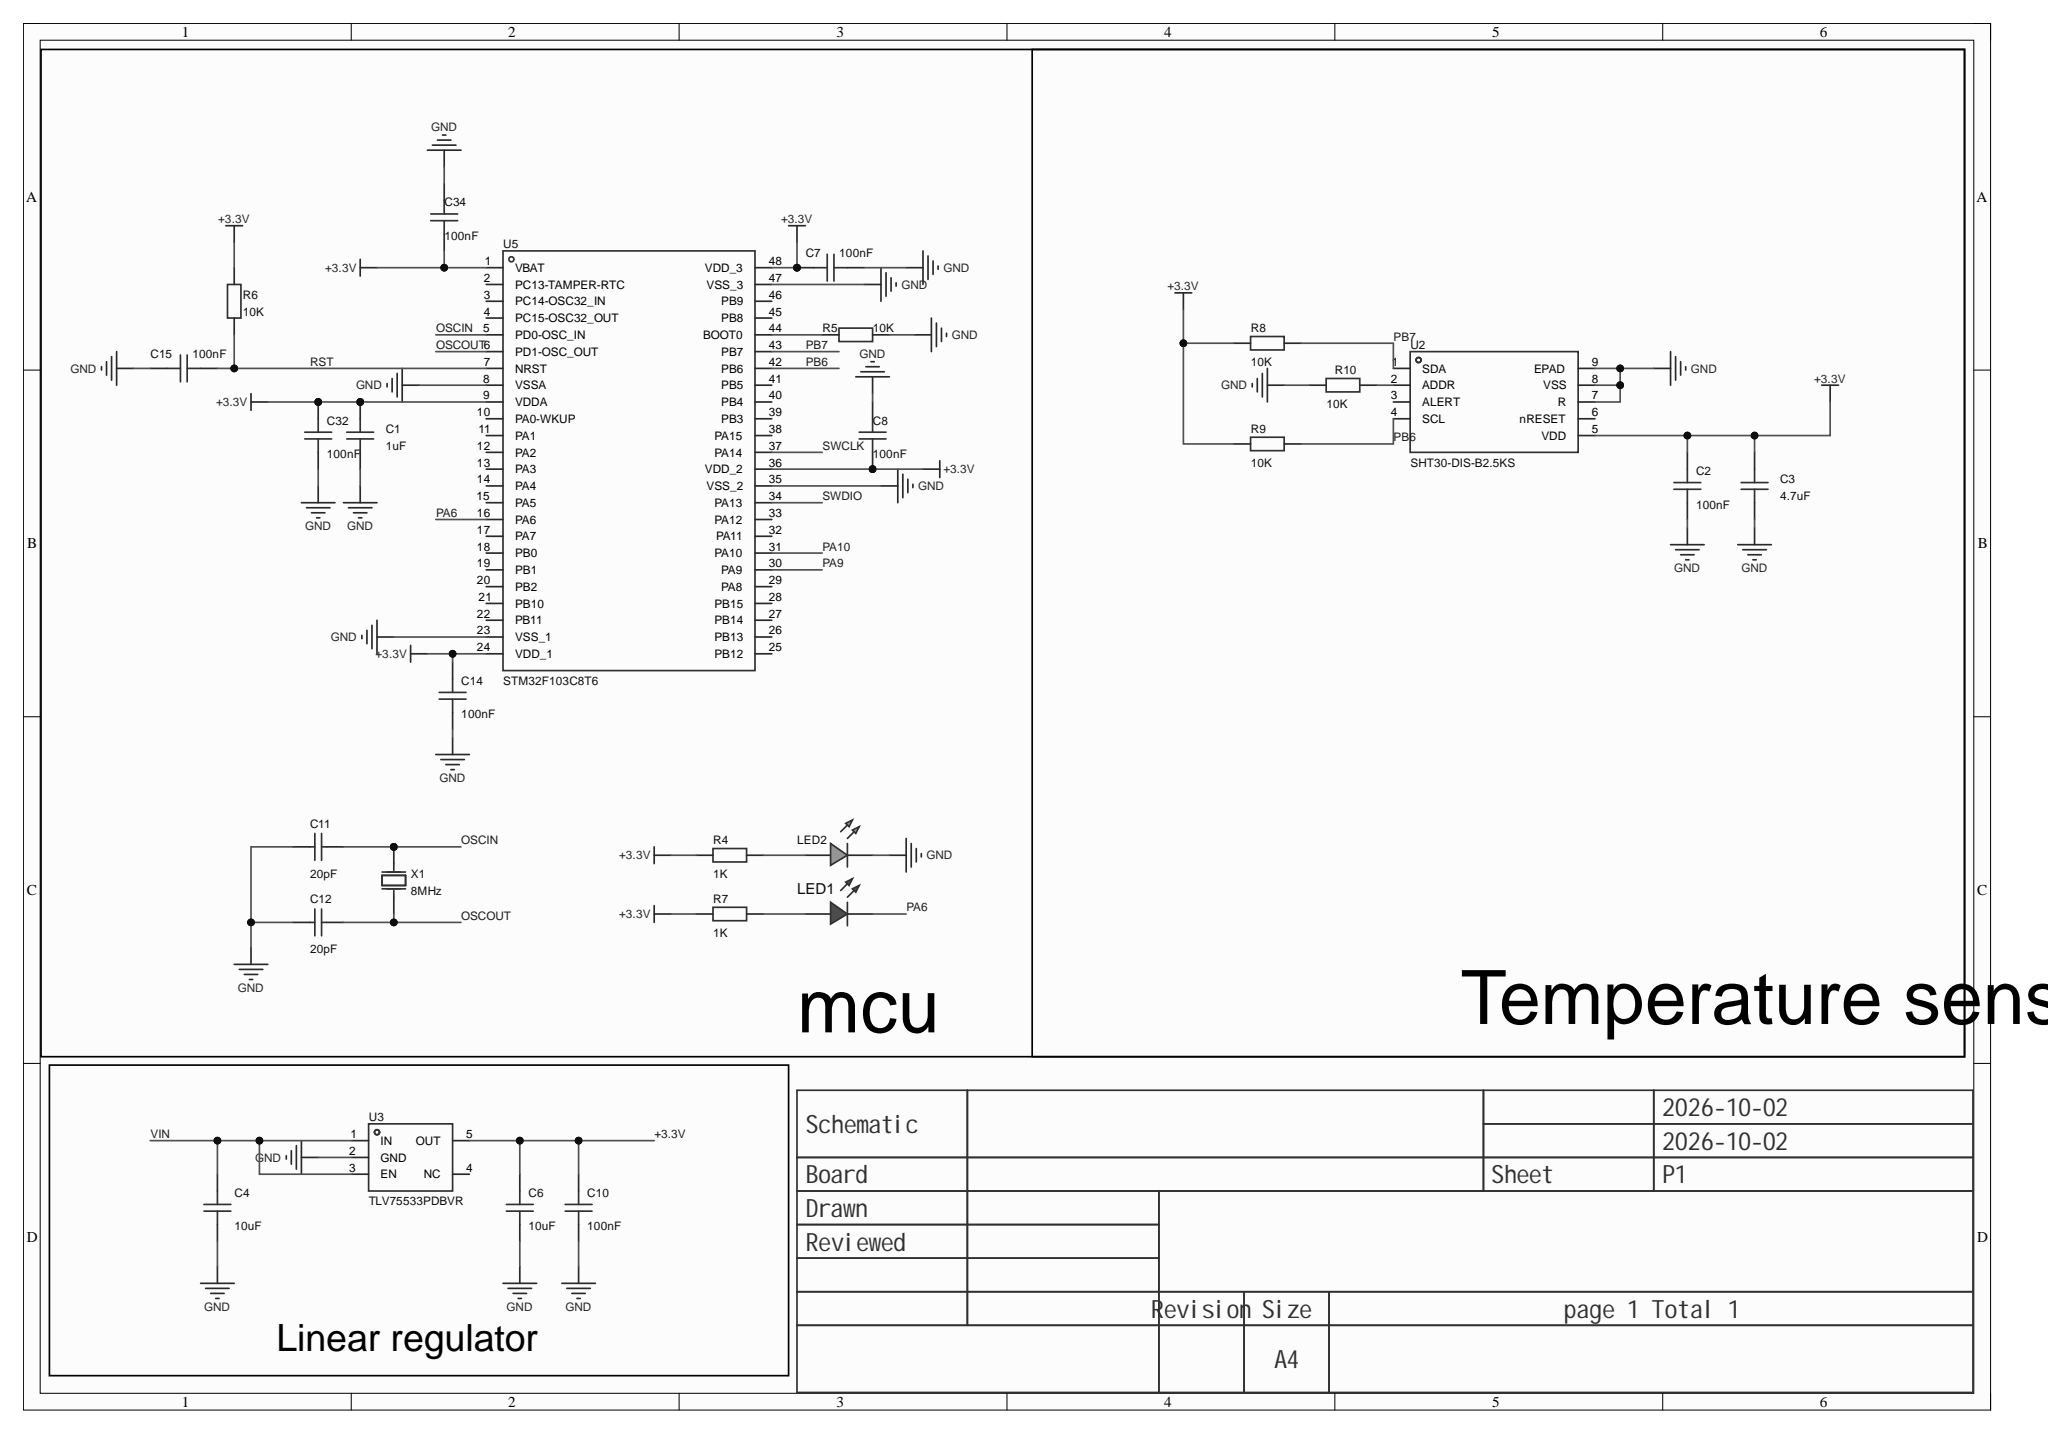Circuit board | Altium Designer | 27 parts | 13 nets
Bill of materials:
Comment,Description,Designator,Footprint,LibRef,Quantity
"1uF","Capacitance:1uF;Accuracy:±10%;Rated voltage:50V;Temperature coefficient:X5R;","C1","C0603","CL10A105KB8NNNC","1"
"100nF","Capacitance:100nF;Accuracy:±10%;Rated voltage:50V;Temperature coefficient:X7R;, [NoValue]","C2, C7, C8, C10, C14, C15, C32, C34","C0603","CGA0603X7R104K500JT, CAP_0603","8"
"4.7uF","Capacitance:4.7uF;Accuracy:±10%;Rated voltage:50V;Temperature coefficient:X7R;","C3","C0805","HGC0805R7475K500NSLJ","1"
"10uF","Capacitance:10uF;Accuracy:±20%;Rated voltage:16V;Temperature coefficient:X5R;","C4, C6","C0603","HGC0603R5106M160NTHJ","2"
"20pF","Capacitance:20pF;Accuracy:±5%;Rated voltage:50V;Temperature coefficient:C0G;","C11, C12","C0603","CL10C200JB8NNNC","2"
"","","LED1, LED2","LED_0603","LED_0603-R, LED_0603-G","2"
"1K","","R4, R7","R0603","Res_0603","2"
"10K","","R5, R6, R8, R9, R10","R0603","Res_0603","5"
"SHT30-DIS-B2.5KS","Temperature range:-40℃~+125℃;Humidity range:0%RH~100%RH;Interface type:I2C;Humidity accuracy:±2%RH;","U2","DFN-8_L2.5-W2.5-P0.50-BL-EP","SHT30-DIS-B2.5KS","1"
"TLV75533PDBVR","Output polarity:Positive;Operating voltage:5.5V;Output voltage:3.3V;Output current:500mA;Power supply rejection ratio (PSRR):46dB@(100kHz);Output type:Fixed;","U3","SOT-23-5_L3.0-W1.7-P0.95-LS2.8-BR","TLV75533PDBVR","1"
"STM32F103C8T6","CPU core:ARM-M3;Max CPU frequency:72MHz;Application field:-;","U5","LQFP-48_L7.0-W7.0-P0.50-LS9.0-BL","STM32F103C8T6","1"
"8MHz","Crystal type:SMD crystal;Frequency:8MHz;Frequency tolerance at room temperature:±10ppm;Load capacitance:20pF;Frequency stability:±20ppm;","X1","CRYSTAL-SMD_L5.0-W3.2","X50328MSB2GI","1"
Netlist (Protel format):
[
C1
C0603
1uF



]
[
C2
C0603
100nF



]
[
C3
C0805
4.7uF



]
[
C4
C0603
10uF



]
[
C6
C0603
10uF



]
[
C7
C0603
100nF



]
[
C8
C0603
100nF



]
[
C10
C0603
100nF



]
[
C11
C0603
20pF



]
[
C12
C0603
20pF



]
[
C14
C0603
100nF



]
[
C15
C0603
100nF



]
[
C32
C0603
100nF



]
[
C34
C0603
100nF



]
[
LED1
LED_0603




]
[
LED2
LED_0603




]
[
R4
R0603
1K



]
[
R5
R0603
10K



]
[
R6
R0603
10K



]
[
R7
R0603
1K



]
[
R8
R0603
10K



]
[
R9
R0603
10K



]
[
R10
R0603
10K



]
[
U2
DFN-8_L2.5-W2.5-P0.50-BL-EP
SHT30-DIS-B2.5KS



]
[
U3
SOT-23-5_L3.0-W1.7-P0.95-LS2.8-BR
TLV75533PDBVR



]
[
U5
LQFP-48_L7.0-W7.0-P0.50-LS9.0-BL
STM32F103C8T6



]
[
X1
CRYSTAL-SMD_L5.0-W3.2
8MHz



]
(
VIN
C4-2
U3-1
U3-3
)
(
RST
C15-1
R6-1
U5-7
)
(
PB7
R8-1
U2-1
U5-43
)
(
PB6
R9-1
U2-4
U5-42
)
(
PA6
LED1-1
U5-16
)
(
OSCOUT
C12-2
U5-6
X1-1
)
(
OSCIN
C11-2
U5-5
X1-2
)
(
NetR10_1
R10-1
U2-2
)
(
NetR5_1
R5-1
U5-44
)
(
NetLED2_2
LED2-2
R4-2
)
(
NetLED1_2
LED1-2
R7-2
)
(
GND
C1-1
C2-2
C3-1
C4-1
C6-2
C7-1
C8-2
C10-1
C11-1
C12-1
C14-2
C15-2
C32-1
C34-2
LED2-1
R5-2
R10-2
U2-7
U2-8
U2-9
U3-2
U5-8
U5-23
U5-35
U5-47
)
(
+3.3V
C1-2
C2-1
C3-2
C6-1
C7-2
C8-1
C10-2
C14-1
C32-2
C34-1
R4-1
R6-2
R7-1
R8-2
R9-2
U2-5
U3-5
U5-1
U5-9
U5-24
U5-36
U5-48
)